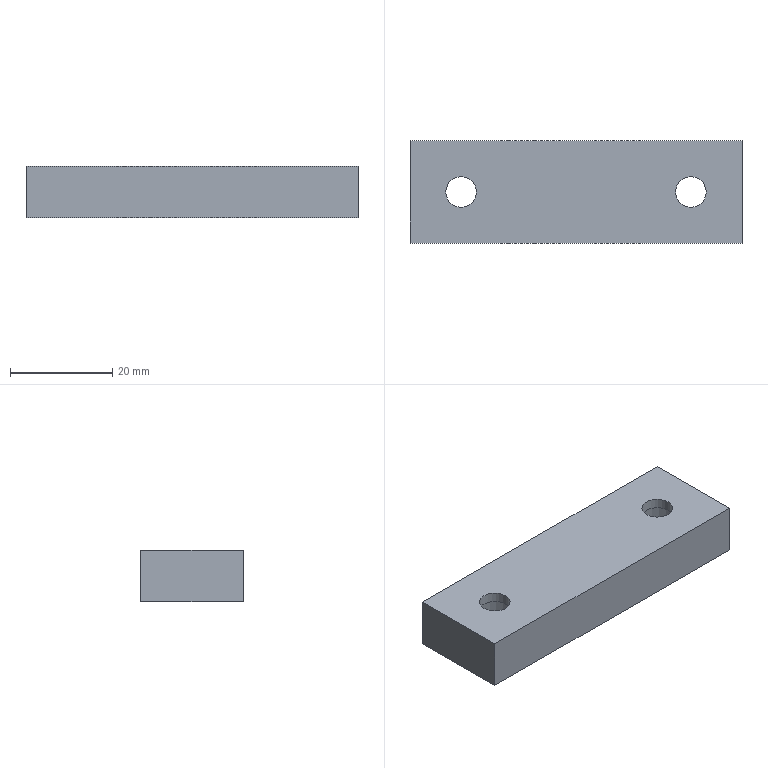Part | STEP file | gslz 2016.10.28-10_id2314_x_t | 1 solid | 12 faces | box 65 x 20 x 10 mm | volume 11366 mm3 | plane 8 | cylinder 4 | commonest cylinder face diameters 6 x2 11 x2
STEP:
#1=CARTESIAN_POINT('',(0.,0.,0.));
#2=DIRECTION('',(0.,0.,1.));
#3=DIRECTION('',(1.,0.,0.));
#4=AXIS2_PLACEMENT_3D('',#1,#2,#3);
#5=CARTESIAN_POINT('',(-56.5,250.,33.));
#6=VERTEX_POINT('',#5);
#7=CARTESIAN_POINT('',(-51.,250.,33.));
#8=DIRECTION('',(0.,0.,1.));
#9=DIRECTION('',(-1.,0.,0.));
#10=AXIS2_PLACEMENT_3D('',#7,#8,#9);
#11=CIRCLE('',#10,5.5);
#12=CARTESIAN_POINT('',(-51.,250.,35.));
#13=DIRECTION('',(0.,0.,-1.));
#14=DIRECTION('',(-1.,0.,0.));
#15=AXIS2_PLACEMENT_3D('',#12,#13,#14);
#16=CYLINDRICAL_SURFACE('',#15,5.5);
#17=CARTESIAN_POINT('',(6.283,2.));
#18=DIRECTION('',(-1.,0.));
#19=VECTOR('',#18,1.);
#20=LINE('',#17,#19);
#21=(GEOMETRIC_REPRESENTATION_CONTEXT(2)PARAMETRIC_REPRESENTATION_CONTEXT()REPRESENTATION_CONTEXT('',''));
#22=DEFINITIONAL_REPRESENTATION('',(#20),#21);
#23=PCURVE('',#16,#22);
#24=CARTESIAN_POINT('',(-13.5,250.,33.));
#25=DIRECTION('',(0.,0.,-1.));
#26=DIRECTION('',(1.,0.,0.));
#27=AXIS2_PLACEMENT_3D('',#24,#25,#26);
#28=PLANE('',#27);
#29=CARTESIAN_POINT('',(-43.,0.));
#30=CARTESIAN_POINT('',(-43.,9.526));
#31=CARTESIAN_POINT('',(-34.75,4.763));
#32=CARTESIAN_POINT('',(-26.5,0.));
#33=CARTESIAN_POINT('',(-34.75,-4.763));
#34=CARTESIAN_POINT('',(-43.,-9.526));
#35=CARTESIAN_POINT('',(-43.,0.));
#36=(BOUNDED_CURVE()B_SPLINE_CURVE(2,(#29,#30,#31,#32,#33,#34,#35),.UNSPECIFIED.,.T.,.F.)B_SPLINE_CURVE_WITH_KNOTS((1,2,2,2,2,1),(-2.094,0.,2.094,4.189,6.283,8.378),.UNSPECIFIED.)CURVE()GEOMETRIC_REPRESENTATION_ITEM()RATIONAL_B_SPLINE_CURVE((1.,0.5,1.,0.5,1.,0.5,1.))REPRESENTATION_ITEM(''));
#37=(GEOMETRIC_REPRESENTATION_CONTEXT(2)PARAMETRIC_REPRESENTATION_CONTEXT()REPRESENTATION_CONTEXT('',''));
#38=DEFINITIONAL_REPRESENTATION('',(#36),#37);
#39=PCURVE('',#28,#38);
#40=SURFACE_CURVE('',#11,(#23,#39),.PCURVE_S1.);
#41=EDGE_CURVE('',#6,#6,#40,.T.);
#42=ORIENTED_EDGE('',*,*,#41,.F.);
#43=CARTESIAN_POINT('',(-56.5,250.,25.));
#44=VERTEX_POINT('',#43);
#45=CARTESIAN_POINT('',(-56.5,250.,33.));
#46=CARTESIAN_POINT('',(-56.5,250.,25.));
#47=B_SPLINE_CURVE_WITH_KNOTS('',1,(#45,#46),.UNSPECIFIED.,.F.,.F.,(2,2),(2.,10.),.PIECEWISE_BEZIER_KNOTS.);
#48=CARTESIAN_POINT('',(6.283,0.));
#49=DIRECTION('',(0.,1.));
#50=VECTOR('',#49,1.);
#51=LINE('',#48,#50);
#52=(GEOMETRIC_REPRESENTATION_CONTEXT(2)PARAMETRIC_REPRESENTATION_CONTEXT()REPRESENTATION_CONTEXT('',''));
#53=DEFINITIONAL_REPRESENTATION('',(#51),#52);
#54=PCURVE('',#16,#53);
#55=CARTESIAN_POINT('',(0.,0.));
#56=DIRECTION('',(0.,1.));
#57=VECTOR('',#56,1.);
#58=LINE('',#55,#57);
#59=(GEOMETRIC_REPRESENTATION_CONTEXT(2)PARAMETRIC_REPRESENTATION_CONTEXT()REPRESENTATION_CONTEXT('',''));
#60=DEFINITIONAL_REPRESENTATION('',(#58),#59);
#61=PCURVE('',#16,#60);
#62=SEAM_CURVE('',#47,(#54,#61),.PCURVE_S1.);
#63=EDGE_CURVE('',#6,#44,#62,.T.);
#64=ORIENTED_EDGE('',*,*,#63,.T.);
#65=CARTESIAN_POINT('',(-45.5,250.,25.));
#66=VERTEX_POINT('',#65);
#67=CARTESIAN_POINT('',(-51.,250.,25.));
#68=DIRECTION('',(0.,0.,1.));
#69=DIRECTION('',(1.,0.,0.));
#70=AXIS2_PLACEMENT_3D('',#67,#68,#69);
#71=CIRCLE('',#70,5.5);
#72=CARTESIAN_POINT('',(9.425,10.));
#73=DIRECTION('',(-1.,0.));
#74=VECTOR('',#73,1.);
#75=LINE('',#72,#74);
#76=(GEOMETRIC_REPRESENTATION_CONTEXT(2)PARAMETRIC_REPRESENTATION_CONTEXT()REPRESENTATION_CONTEXT('',''));
#77=DEFINITIONAL_REPRESENTATION('',(#75),#76);
#78=PCURVE('',#16,#77);
#79=CARTESIAN_POINT('',(-98.5,250.,25.));
#80=DIRECTION('',(0.,0.,1.));
#81=DIRECTION('',(1.,0.,0.));
#82=AXIS2_PLACEMENT_3D('',#79,#80,#81);
#83=PLANE('',#82);
#84=CARTESIAN_POINT('',(47.5,0.));
#85=DIRECTION('',(1.,0.));
#86=AXIS2_PLACEMENT_2D('',#84,#85);
#87=CIRCLE('',#86,5.5);
#88=(GEOMETRIC_REPRESENTATION_CONTEXT(2)PARAMETRIC_REPRESENTATION_CONTEXT()REPRESENTATION_CONTEXT('',''));
#89=DEFINITIONAL_REPRESENTATION('',(#87),#88);
#90=PCURVE('',#83,#89);
#91=SURFACE_CURVE('',#71,(#78,#90),.PCURVE_S1.);
#92=EDGE_CURVE('',#44,#66,#91,.T.);
#93=ORIENTED_EDGE('',*,*,#92,.T.);
#94=CARTESIAN_POINT('',(-51.,250.,25.));
#95=DIRECTION('',(0.,0.,1.));
#96=DIRECTION('',(1.,0.,0.));
#97=AXIS2_PLACEMENT_3D('',#94,#95,#96);
#98=CIRCLE('',#97,5.5);
#99=CARTESIAN_POINT('',(3.142,10.));
#100=DIRECTION('',(-1.,0.));
#101=VECTOR('',#100,1.);
#102=LINE('',#99,#101);
#103=(GEOMETRIC_REPRESENTATION_CONTEXT(2)PARAMETRIC_REPRESENTATION_CONTEXT()REPRESENTATION_CONTEXT('',''));
#104=DEFINITIONAL_REPRESENTATION('',(#102),#103);
#105=PCURVE('',#16,#104);
#106=CARTESIAN_POINT('',(47.5,0.));
#107=DIRECTION('',(1.,0.));
#108=AXIS2_PLACEMENT_2D('',#106,#107);
#109=CIRCLE('',#108,5.5);
#110=(GEOMETRIC_REPRESENTATION_CONTEXT(2)PARAMETRIC_REPRESENTATION_CONTEXT()REPRESENTATION_CONTEXT('',''));
#111=DEFINITIONAL_REPRESENTATION('',(#109),#110);
#112=PCURVE('',#83,#111);
#113=SURFACE_CURVE('',#98,(#105,#112),.PCURVE_S1.);
#114=EDGE_CURVE('',#66,#44,#113,.T.);
#115=ORIENTED_EDGE('',*,*,#114,.T.);
#116=ORIENTED_EDGE('',*,*,#63,.F.);
#117=EDGE_LOOP('',(#42,#64,#93,#115,#116));
#118=FACE_BOUND('',#117,.F.);
#119=ADVANCED_FACE('',(#118),#16,.F.);
#120=CARTESIAN_POINT('',(-61.,260.,35.));
#121=VERTEX_POINT('',#120);
#122=CARTESIAN_POINT('',(-61.,260.,25.));
#123=VERTEX_POINT('',#122);
#124=CARTESIAN_POINT('',(-61.,260.,35.));
#125=DIRECTION('',(0.,0.,-1.));
#126=VECTOR('',#125,1.);
#127=LINE('',#124,#126);
#128=CARTESIAN_POINT('',(21.5,260.,35.));
#129=DIRECTION('',(0.,-1.,0.));
#130=DIRECTION('',(0.,0.,-1.));
#131=AXIS2_PLACEMENT_3D('',#128,#129,#130);
#132=PLANE('',#131);
#133=CARTESIAN_POINT('',(0.,-82.5));
#134=DIRECTION('',(1.,0.));
#135=VECTOR('',#134,1.);
#136=LINE('',#133,#135);
#137=(GEOMETRIC_REPRESENTATION_CONTEXT(2)PARAMETRIC_REPRESENTATION_CONTEXT()REPRESENTATION_CONTEXT('',''));
#138=DEFINITIONAL_REPRESENTATION('',(#136),#137);
#139=PCURVE('',#132,#138);
#140=CARTESIAN_POINT('',(-61.,262.5,35.));
#141=DIRECTION('',(1.,0.,0.));
#142=DIRECTION('',(0.,0.,-1.));
#143=AXIS2_PLACEMENT_3D('',#140,#141,#142);
#144=PLANE('',#143);
#145=CARTESIAN_POINT('',(0.,-2.5));
#146=DIRECTION('',(1.,0.));
#147=VECTOR('',#146,1.);
#148=LINE('',#145,#147);
#149=(GEOMETRIC_REPRESENTATION_CONTEXT(2)PARAMETRIC_REPRESENTATION_CONTEXT()REPRESENTATION_CONTEXT('',''));
#150=DEFINITIONAL_REPRESENTATION('',(#148),#149);
#151=PCURVE('',#144,#150);
#152=SURFACE_CURVE('',#127,(#139,#151),.PCURVE_S1.);
#153=EDGE_CURVE('',#121,#123,#152,.T.);
#154=ORIENTED_EDGE('',*,*,#153,.F.);
#155=CARTESIAN_POINT('',(4.,260.,35.));
#156=VERTEX_POINT('',#155);
#157=CARTESIAN_POINT('',(-98.5,260.,35.));
#158=DIRECTION('',(-1.,0.,0.));
#159=VECTOR('',#158,1.);
#160=LINE('',#157,#159);
#161=CARTESIAN_POINT('',(0.,-120.));
#162=DIRECTION('',(0.,-1.));
#163=VECTOR('',#162,1.);
#164=LINE('',#161,#163);
#165=(GEOMETRIC_REPRESENTATION_CONTEXT(2)PARAMETRIC_REPRESENTATION_CONTEXT()REPRESENTATION_CONTEXT('',''));
#166=DEFINITIONAL_REPRESENTATION('',(#164),#165);
#167=PCURVE('',#132,#166);
#168=CARTESIAN_POINT('',(-98.5,250.,35.));
#169=DIRECTION('',(0.,0.,1.));
#170=DIRECTION('',(1.,0.,0.));
#171=AXIS2_PLACEMENT_3D('',#168,#169,#170);
#172=PLANE('',#171);
#173=CARTESIAN_POINT('',(0.,10.));
#174=DIRECTION('',(-1.,0.));
#175=VECTOR('',#174,1.);
#176=LINE('',#173,#175);
#177=(GEOMETRIC_REPRESENTATION_CONTEXT(2)PARAMETRIC_REPRESENTATION_CONTEXT()REPRESENTATION_CONTEXT('',''));
#178=DEFINITIONAL_REPRESENTATION('',(#176),#177);
#179=PCURVE('',#172,#178);
#180=SURFACE_CURVE('',#160,(#167,#179),.PCURVE_S1.);
#181=EDGE_CURVE('',#156,#121,#180,.T.);
#182=ORIENTED_EDGE('',*,*,#181,.F.);
#183=CARTESIAN_POINT('',(4.,260.,25.));
#184=VERTEX_POINT('',#183);
#185=CARTESIAN_POINT('',(4.,260.,35.));
#186=DIRECTION('',(0.,0.,-1.));
#187=VECTOR('',#186,1.);
#188=LINE('',#185,#187);
#189=CARTESIAN_POINT('',(0.,-17.5));
#190=DIRECTION('',(1.,0.));
#191=VECTOR('',#190,1.);
#192=LINE('',#189,#191);
#193=(GEOMETRIC_REPRESENTATION_CONTEXT(2)PARAMETRIC_REPRESENTATION_CONTEXT()REPRESENTATION_CONTEXT('',''));
#194=DEFINITIONAL_REPRESENTATION('',(#192),#193);
#195=PCURVE('',#132,#194);
#196=CARTESIAN_POINT('',(4.,237.5,35.));
#197=DIRECTION('',(-1.,0.,0.));
#198=DIRECTION('',(0.,0.,1.));
#199=AXIS2_PLACEMENT_3D('',#196,#197,#198);
#200=PLANE('',#199);
#201=CARTESIAN_POINT('',(0.,22.5));
#202=DIRECTION('',(-1.,0.));
#203=VECTOR('',#202,1.);
#204=LINE('',#201,#203);
#205=(GEOMETRIC_REPRESENTATION_CONTEXT(2)PARAMETRIC_REPRESENTATION_CONTEXT()REPRESENTATION_CONTEXT('',''));
#206=DEFINITIONAL_REPRESENTATION('',(#204),#205);
#207=PCURVE('',#200,#206);
#208=SURFACE_CURVE('',#188,(#195,#207),.PCURVE_S1.);
#209=EDGE_CURVE('',#156,#184,#208,.T.);
#210=ORIENTED_EDGE('',*,*,#209,.T.);
#211=CARTESIAN_POINT('',(-98.5,260.,25.));
#212=DIRECTION('',(-1.,0.,0.));
#213=VECTOR('',#212,1.);
#214=LINE('',#211,#213);
#215=CARTESIAN_POINT('',(10.,-120.));
#216=DIRECTION('',(0.,-1.));
#217=VECTOR('',#216,1.);
#218=LINE('',#215,#217);
#219=(GEOMETRIC_REPRESENTATION_CONTEXT(2)PARAMETRIC_REPRESENTATION_CONTEXT()REPRESENTATION_CONTEXT('',''));
#220=DEFINITIONAL_REPRESENTATION('',(#218),#219);
#221=PCURVE('',#132,#220);
#222=CARTESIAN_POINT('',(0.,10.));
#223=DIRECTION('',(-1.,0.));
#224=VECTOR('',#223,1.);
#225=LINE('',#222,#224);
#226=(GEOMETRIC_REPRESENTATION_CONTEXT(2)PARAMETRIC_REPRESENTATION_CONTEXT()REPRESENTATION_CONTEXT('',''));
#227=DEFINITIONAL_REPRESENTATION('',(#225),#226);
#228=PCURVE('',#83,#227);
#229=SURFACE_CURVE('',#214,(#221,#228),.PCURVE_S1.);
#230=EDGE_CURVE('',#184,#123,#229,.T.);
#231=ORIENTED_EDGE('',*,*,#230,.T.);
#232=EDGE_LOOP('',(#154,#182,#210,#231));
#233=FACE_BOUND('',#232,.T.);
#234=ADVANCED_FACE('',(#233),#132,.F.);
#235=ORIENTED_EDGE('',*,*,#209,.F.);
#236=CARTESIAN_POINT('',(4.,240.,35.));
#237=VERTEX_POINT('',#236);
#238=CARTESIAN_POINT('',(4.,237.5,35.));
#239=DIRECTION('',(0.,1.,0.));
#240=VECTOR('',#239,1.);
#241=LINE('',#238,#240);
#242=CARTESIAN_POINT('',(0.,0.));
#243=DIRECTION('',(0.,1.));
#244=VECTOR('',#243,1.);
#245=LINE('',#242,#244);
#246=(GEOMETRIC_REPRESENTATION_CONTEXT(2)PARAMETRIC_REPRESENTATION_CONTEXT()REPRESENTATION_CONTEXT('',''));
#247=DEFINITIONAL_REPRESENTATION('',(#245),#246);
#248=PCURVE('',#200,#247);
#249=CARTESIAN_POINT('',(102.5,-12.5));
#250=DIRECTION('',(0.,1.));
#251=VECTOR('',#250,1.);
#252=LINE('',#249,#251);
#253=(GEOMETRIC_REPRESENTATION_CONTEXT(2)PARAMETRIC_REPRESENTATION_CONTEXT()REPRESENTATION_CONTEXT('',''));
#254=DEFINITIONAL_REPRESENTATION('',(#252),#253);
#255=PCURVE('',#172,#254);
#256=SURFACE_CURVE('',#241,(#248,#255),.PCURVE_S1.);
#257=EDGE_CURVE('',#237,#156,#256,.T.);
#258=ORIENTED_EDGE('',*,*,#257,.F.);
#259=CARTESIAN_POINT('',(4.,240.,25.));
#260=VERTEX_POINT('',#259);
#261=CARTESIAN_POINT('',(4.,240.,35.));
#262=DIRECTION('',(0.,0.,-1.));
#263=VECTOR('',#262,1.);
#264=LINE('',#261,#263);
#265=CARTESIAN_POINT('',(0.,2.5));
#266=DIRECTION('',(-1.,0.));
#267=VECTOR('',#266,1.);
#268=LINE('',#265,#267);
#269=(GEOMETRIC_REPRESENTATION_CONTEXT(2)PARAMETRIC_REPRESENTATION_CONTEXT()REPRESENTATION_CONTEXT('',''));
#270=DEFINITIONAL_REPRESENTATION('',(#268),#269);
#271=PCURVE('',#200,#270);
#272=CARTESIAN_POINT('',(-108.5,240.,35.));
#273=DIRECTION('',(0.,1.,0.));
#274=DIRECTION('',(0.,0.,1.));
#275=AXIS2_PLACEMENT_3D('',#272,#273,#274);
#276=PLANE('',#275);
#277=CARTESIAN_POINT('',(0.,112.5));
#278=DIRECTION('',(-1.,0.));
#279=VECTOR('',#278,1.);
#280=LINE('',#277,#279);
#281=(GEOMETRIC_REPRESENTATION_CONTEXT(2)PARAMETRIC_REPRESENTATION_CONTEXT()REPRESENTATION_CONTEXT('',''));
#282=DEFINITIONAL_REPRESENTATION('',(#280),#281);
#283=PCURVE('',#276,#282);
#284=SURFACE_CURVE('',#264,(#271,#283),.PCURVE_S1.);
#285=EDGE_CURVE('',#237,#260,#284,.T.);
#286=ORIENTED_EDGE('',*,*,#285,.T.);
#287=CARTESIAN_POINT('',(4.,237.5,25.));
#288=DIRECTION('',(0.,1.,0.));
#289=VECTOR('',#288,1.);
#290=LINE('',#287,#289);
#291=CARTESIAN_POINT('',(-10.,0.));
#292=DIRECTION('',(0.,1.));
#293=VECTOR('',#292,1.);
#294=LINE('',#291,#293);
#295=(GEOMETRIC_REPRESENTATION_CONTEXT(2)PARAMETRIC_REPRESENTATION_CONTEXT()REPRESENTATION_CONTEXT('',''));
#296=DEFINITIONAL_REPRESENTATION('',(#294),#295);
#297=PCURVE('',#200,#296);
#298=CARTESIAN_POINT('',(102.5,-12.5));
#299=DIRECTION('',(0.,1.));
#300=VECTOR('',#299,1.);
#301=LINE('',#298,#300);
#302=(GEOMETRIC_REPRESENTATION_CONTEXT(2)PARAMETRIC_REPRESENTATION_CONTEXT()REPRESENTATION_CONTEXT('',''));
#303=DEFINITIONAL_REPRESENTATION('',(#301),#302);
#304=PCURVE('',#83,#303);
#305=SURFACE_CURVE('',#290,(#297,#304),.PCURVE_S1.);
#306=EDGE_CURVE('',#260,#184,#305,.T.);
#307=ORIENTED_EDGE('',*,*,#306,.T.);
#308=EDGE_LOOP('',(#235,#258,#286,#307));
#309=FACE_BOUND('',#308,.T.);
#310=ADVANCED_FACE('',(#309),#200,.F.);
#311=ORIENTED_EDGE('',*,*,#285,.F.);
#312=CARTESIAN_POINT('',(-61.,240.,35.));
#313=VERTEX_POINT('',#312);
#314=CARTESIAN_POINT('',(-98.5,240.,35.));
#315=DIRECTION('',(1.,0.,0.));
#316=VECTOR('',#315,1.);
#317=LINE('',#314,#316);
#318=CARTESIAN_POINT('',(0.,10.));
#319=DIRECTION('',(0.,1.));
#320=VECTOR('',#319,1.);
#321=LINE('',#318,#320);
#322=(GEOMETRIC_REPRESENTATION_CONTEXT(2)PARAMETRIC_REPRESENTATION_CONTEXT()REPRESENTATION_CONTEXT('',''));
#323=DEFINITIONAL_REPRESENTATION('',(#321),#322);
#324=PCURVE('',#276,#323);
#325=CARTESIAN_POINT('',(0.,-10.));
#326=DIRECTION('',(1.,0.));
#327=VECTOR('',#326,1.);
#328=LINE('',#325,#327);
#329=(GEOMETRIC_REPRESENTATION_CONTEXT(2)PARAMETRIC_REPRESENTATION_CONTEXT()REPRESENTATION_CONTEXT('',''));
#330=DEFINITIONAL_REPRESENTATION('',(#328),#329);
#331=PCURVE('',#172,#330);
#332=SURFACE_CURVE('',#317,(#324,#331),.PCURVE_S1.);
#333=EDGE_CURVE('',#313,#237,#332,.T.);
#334=ORIENTED_EDGE('',*,*,#333,.F.);
#335=CARTESIAN_POINT('',(-61.,240.,25.));
#336=VERTEX_POINT('',#335);
#337=CARTESIAN_POINT('',(-61.,240.,35.));
#338=DIRECTION('',(0.,0.,-1.));
#339=VECTOR('',#338,1.);
#340=LINE('',#337,#339);
#341=CARTESIAN_POINT('',(0.,47.5));
#342=DIRECTION('',(-1.,0.));
#343=VECTOR('',#342,1.);
#344=LINE('',#341,#343);
#345=(GEOMETRIC_REPRESENTATION_CONTEXT(2)PARAMETRIC_REPRESENTATION_CONTEXT()REPRESENTATION_CONTEXT('',''));
#346=DEFINITIONAL_REPRESENTATION('',(#344),#345);
#347=PCURVE('',#276,#346);
#348=CARTESIAN_POINT('',(0.,-22.5));
#349=DIRECTION('',(1.,0.));
#350=VECTOR('',#349,1.);
#351=LINE('',#348,#350);
#352=(GEOMETRIC_REPRESENTATION_CONTEXT(2)PARAMETRIC_REPRESENTATION_CONTEXT()REPRESENTATION_CONTEXT('',''));
#353=DEFINITIONAL_REPRESENTATION('',(#351),#352);
#354=PCURVE('',#144,#353);
#355=SURFACE_CURVE('',#340,(#347,#354),.PCURVE_S1.);
#356=EDGE_CURVE('',#313,#336,#355,.T.);
#357=ORIENTED_EDGE('',*,*,#356,.T.);
#358=CARTESIAN_POINT('',(-98.5,240.,25.));
#359=DIRECTION('',(1.,0.,0.));
#360=VECTOR('',#359,1.);
#361=LINE('',#358,#360);
#362=CARTESIAN_POINT('',(-10.,10.));
#363=DIRECTION('',(0.,1.));
#364=VECTOR('',#363,1.);
#365=LINE('',#362,#364);
#366=(GEOMETRIC_REPRESENTATION_CONTEXT(2)PARAMETRIC_REPRESENTATION_CONTEXT()REPRESENTATION_CONTEXT('',''));
#367=DEFINITIONAL_REPRESENTATION('',(#365),#366);
#368=PCURVE('',#276,#367);
#369=CARTESIAN_POINT('',(0.,-10.));
#370=DIRECTION('',(1.,0.));
#371=VECTOR('',#370,1.);
#372=LINE('',#369,#371);
#373=(GEOMETRIC_REPRESENTATION_CONTEXT(2)PARAMETRIC_REPRESENTATION_CONTEXT()REPRESENTATION_CONTEXT('',''));
#374=DEFINITIONAL_REPRESENTATION('',(#372),#373);
#375=PCURVE('',#83,#374);
#376=SURFACE_CURVE('',#361,(#368,#375),.PCURVE_S1.);
#377=EDGE_CURVE('',#336,#260,#376,.T.);
#378=ORIENTED_EDGE('',*,*,#377,.T.);
#379=EDGE_LOOP('',(#311,#334,#357,#378));
#380=FACE_BOUND('',#379,.T.);
#381=ADVANCED_FACE('',(#380),#276,.F.);
#382=ORIENTED_EDGE('',*,*,#356,.F.);
#383=CARTESIAN_POINT('',(-61.,262.5,35.));
#384=DIRECTION('',(0.,-1.,0.));
#385=VECTOR('',#384,1.);
#386=LINE('',#383,#385);
#387=CARTESIAN_POINT('',(0.,0.));
#388=DIRECTION('',(0.,-1.));
#389=VECTOR('',#388,1.);
#390=LINE('',#387,#389);
#391=(GEOMETRIC_REPRESENTATION_CONTEXT(2)PARAMETRIC_REPRESENTATION_CONTEXT()REPRESENTATION_CONTEXT('',''));
#392=DEFINITIONAL_REPRESENTATION('',(#390),#391);
#393=PCURVE('',#144,#392);
#394=CARTESIAN_POINT('',(37.5,12.5));
#395=DIRECTION('',(0.,-1.));
#396=VECTOR('',#395,1.);
#397=LINE('',#394,#396);
#398=(GEOMETRIC_REPRESENTATION_CONTEXT(2)PARAMETRIC_REPRESENTATION_CONTEXT()REPRESENTATION_CONTEXT('',''));
#399=DEFINITIONAL_REPRESENTATION('',(#397),#398);
#400=PCURVE('',#172,#399);
#401=SURFACE_CURVE('',#386,(#393,#400),.PCURVE_S1.);
#402=EDGE_CURVE('',#121,#313,#401,.T.);
#403=ORIENTED_EDGE('',*,*,#402,.F.);
#404=ORIENTED_EDGE('',*,*,#153,.T.);
#405=CARTESIAN_POINT('',(-61.,262.5,25.));
#406=DIRECTION('',(0.,-1.,0.));
#407=VECTOR('',#406,1.);
#408=LINE('',#405,#407);
#409=CARTESIAN_POINT('',(10.,0.));
#410=DIRECTION('',(0.,-1.));
#411=VECTOR('',#410,1.);
#412=LINE('',#409,#411);
#413=(GEOMETRIC_REPRESENTATION_CONTEXT(2)PARAMETRIC_REPRESENTATION_CONTEXT()REPRESENTATION_CONTEXT('',''));
#414=DEFINITIONAL_REPRESENTATION('',(#412),#413);
#415=PCURVE('',#144,#414);
#416=CARTESIAN_POINT('',(37.5,12.5));
#417=DIRECTION('',(0.,-1.));
#418=VECTOR('',#417,1.);
#419=LINE('',#416,#418);
#420=(GEOMETRIC_REPRESENTATION_CONTEXT(2)PARAMETRIC_REPRESENTATION_CONTEXT()REPRESENTATION_CONTEXT('',''));
#421=DEFINITIONAL_REPRESENTATION('',(#419),#420);
#422=PCURVE('',#83,#421);
#423=SURFACE_CURVE('',#408,(#415,#422),.PCURVE_S1.);
#424=EDGE_CURVE('',#123,#336,#423,.T.);
#425=ORIENTED_EDGE('',*,*,#424,.T.);
#426=EDGE_LOOP('',(#382,#403,#404,#425));
#427=FACE_BOUND('',#426,.T.);
#428=ADVANCED_FACE('',(#427),#144,.F.);
#429=ORIENTED_EDGE('',*,*,#424,.F.);
#430=ORIENTED_EDGE('',*,*,#230,.F.);
#431=ORIENTED_EDGE('',*,*,#306,.F.);
#432=ORIENTED_EDGE('',*,*,#377,.F.);
#433=EDGE_LOOP('',(#429,#430,#431,#432));
#434=FACE_BOUND('',#433,.T.);
#435=ORIENTED_EDGE('',*,*,#114,.T.);
#436=ORIENTED_EDGE('',*,*,#92,.T.);
#437=EDGE_LOOP('',(#435,#436));
#438=FACE_BOUND('',#437,.T.);
#439=CARTESIAN_POINT('',(-0.5,250.,25.));
#440=VERTEX_POINT('',#439);
#441=CARTESIAN_POINT('',(-11.5,250.,25.));
#442=VERTEX_POINT('',#441);
#443=CARTESIAN_POINT('',(-6.,250.,25.));
#444=DIRECTION('',(0.,0.,1.));
#445=DIRECTION('',(1.,0.,0.));
#446=AXIS2_PLACEMENT_3D('',#443,#444,#445);
#447=CIRCLE('',#446,5.5);
#448=CARTESIAN_POINT('',(92.5,0.));
#449=DIRECTION('',(1.,0.));
#450=AXIS2_PLACEMENT_2D('',#448,#449);
#451=CIRCLE('',#450,5.5);
#452=(GEOMETRIC_REPRESENTATION_CONTEXT(2)PARAMETRIC_REPRESENTATION_CONTEXT()REPRESENTATION_CONTEXT('',''));
#453=DEFINITIONAL_REPRESENTATION('',(#451),#452);
#454=PCURVE('',#83,#453);
#455=CARTESIAN_POINT('',(-6.,250.,35.));
#456=DIRECTION('',(0.,0.,-1.));
#457=DIRECTION('',(-1.,0.,0.));
#458=AXIS2_PLACEMENT_3D('',#455,#456,#457);
#459=CYLINDRICAL_SURFACE('',#458,5.5);
#460=CARTESIAN_POINT('',(3.142,10.));
#461=DIRECTION('',(-1.,0.));
#462=VECTOR('',#461,1.);
#463=LINE('',#460,#462);
#464=(GEOMETRIC_REPRESENTATION_CONTEXT(2)PARAMETRIC_REPRESENTATION_CONTEXT()REPRESENTATION_CONTEXT('',''));
#465=DEFINITIONAL_REPRESENTATION('',(#463),#464);
#466=PCURVE('',#459,#465);
#467=SURFACE_CURVE('',#447,(#454,#466),.PCURVE_S1.);
#468=EDGE_CURVE('',#440,#442,#467,.T.);
#469=ORIENTED_EDGE('',*,*,#468,.T.);
#470=CARTESIAN_POINT('',(-6.,250.,25.));
#471=DIRECTION('',(0.,0.,1.));
#472=DIRECTION('',(1.,0.,0.));
#473=AXIS2_PLACEMENT_3D('',#470,#471,#472);
#474=CIRCLE('',#473,5.5);
#475=CARTESIAN_POINT('',(92.5,0.));
#476=DIRECTION('',(1.,0.));
#477=AXIS2_PLACEMENT_2D('',#475,#476);
#478=CIRCLE('',#477,5.5);
#479=(GEOMETRIC_REPRESENTATION_CONTEXT(2)PARAMETRIC_REPRESENTATION_CONTEXT()REPRESENTATION_CONTEXT('',''));
#480=DEFINITIONAL_REPRESENTATION('',(#478),#479);
#481=PCURVE('',#83,#480);
#482=CARTESIAN_POINT('',(9.425,10.));
#483=DIRECTION('',(-1.,0.));
#484=VECTOR('',#483,1.);
#485=LINE('',#482,#484);
#486=(GEOMETRIC_REPRESENTATION_CONTEXT(2)PARAMETRIC_REPRESENTATION_CONTEXT()REPRESENTATION_CONTEXT('',''));
#487=DEFINITIONAL_REPRESENTATION('',(#485),#486);
#488=PCURVE('',#459,#487);
#489=SURFACE_CURVE('',#474,(#481,#488),.PCURVE_S1.);
#490=EDGE_CURVE('',#442,#440,#489,.T.);
#491=ORIENTED_EDGE('',*,*,#490,.T.);
#492=EDGE_LOOP('',(#469,#491));
#493=FACE_BOUND('',#492,.T.);
#494=ADVANCED_FACE('',(#434,#438,#493),#83,.F.);
#495=CARTESIAN_POINT('',(-11.5,250.,33.));
#496=VERTEX_POINT('',#495);
#497=CARTESIAN_POINT('',(-6.,250.,33.));
#498=DIRECTION('',(0.,0.,1.));
#499=DIRECTION('',(-1.,0.,0.));
#500=AXIS2_PLACEMENT_3D('',#497,#498,#499);
#501=CIRCLE('',#500,5.5);
#502=CARTESIAN_POINT('',(6.283,2.));
#503=DIRECTION('',(-1.,0.));
#504=VECTOR('',#503,1.);
#505=LINE('',#502,#504);
#506=(GEOMETRIC_REPRESENTATION_CONTEXT(2)PARAMETRIC_REPRESENTATION_CONTEXT()REPRESENTATION_CONTEXT('',''));
#507=DEFINITIONAL_REPRESENTATION('',(#505),#506);
#508=PCURVE('',#459,#507);
#509=CARTESIAN_POINT('',(-43.5,250.,33.));
#510=DIRECTION('',(0.,0.,-1.));
#511=DIRECTION('',(1.,0.,0.));
#512=AXIS2_PLACEMENT_3D('',#509,#510,#511);
#513=PLANE('',#512);
#514=CARTESIAN_POINT('',(32.,0.));
#515=CARTESIAN_POINT('',(32.,9.526));
#516=CARTESIAN_POINT('',(40.25,4.763));
#517=CARTESIAN_POINT('',(48.5,0.));
#518=CARTESIAN_POINT('',(40.25,-4.763));
#519=CARTESIAN_POINT('',(32.,-9.526));
#520=CARTESIAN_POINT('',(32.,0.));
#521=(BOUNDED_CURVE()B_SPLINE_CURVE(2,(#514,#515,#516,#517,#518,#519,#520),.UNSPECIFIED.,.T.,.F.)B_SPLINE_CURVE_WITH_KNOTS((1,2,2,2,2,1),(-2.094,0.,2.094,4.189,6.283,8.378),.UNSPECIFIED.)CURVE()GEOMETRIC_REPRESENTATION_ITEM()RATIONAL_B_SPLINE_CURVE((1.,0.5,1.,0.5,1.,0.5,1.))REPRESENTATION_ITEM(''));
#522=(GEOMETRIC_REPRESENTATION_CONTEXT(2)PARAMETRIC_REPRESENTATION_CONTEXT()REPRESENTATION_CONTEXT('',''));
#523=DEFINITIONAL_REPRESENTATION('',(#521),#522);
#524=PCURVE('',#513,#523);
#525=SURFACE_CURVE('',#501,(#508,#524),.PCURVE_S1.);
#526=EDGE_CURVE('',#496,#496,#525,.T.);
#527=ORIENTED_EDGE('',*,*,#526,.F.);
#528=CARTESIAN_POINT('',(-11.5,250.,33.));
#529=CARTESIAN_POINT('',(-11.5,250.,25.));
#530=B_SPLINE_CURVE_WITH_KNOTS('',1,(#528,#529),.UNSPECIFIED.,.F.,.F.,(2,2),(2.,10.),.PIECEWISE_BEZIER_KNOTS.);
#531=CARTESIAN_POINT('',(6.283,0.));
#532=DIRECTION('',(0.,1.));
#533=VECTOR('',#532,1.);
#534=LINE('',#531,#533);
#535=(GEOMETRIC_REPRESENTATION_CONTEXT(2)PARAMETRIC_REPRESENTATION_CONTEXT()REPRESENTATION_CONTEXT('',''));
#536=DEFINITIONAL_REPRESENTATION('',(#534),#535);
#537=PCURVE('',#459,#536);
#538=CARTESIAN_POINT('',(0.,0.));
#539=DIRECTION('',(0.,1.));
#540=VECTOR('',#539,1.);
#541=LINE('',#538,#540);
#542=(GEOMETRIC_REPRESENTATION_CONTEXT(2)PARAMETRIC_REPRESENTATION_CONTEXT()REPRESENTATION_CONTEXT('',''));
#543=DEFINITIONAL_REPRESENTATION('',(#541),#542);
#544=PCURVE('',#459,#543);
#545=SEAM_CURVE('',#530,(#537,#544),.PCURVE_S1.);
#546=EDGE_CURVE('',#496,#442,#545,.T.);
#547=ORIENTED_EDGE('',*,*,#546,.T.);
#548=ORIENTED_EDGE('',*,*,#490,.T.);
#549=ORIENTED_EDGE('',*,*,#468,.T.);
#550=ORIENTED_EDGE('',*,*,#546,.F.);
#551=EDGE_LOOP('',(#527,#547,#548,#549,#550));
#552=FACE_BOUND('',#551,.F.);
#553=ADVANCED_FACE('',(#552),#459,.F.);
#554=CARTESIAN_POINT('',(-9.,250.,33.));
#555=VERTEX_POINT('',#554);
#556=CARTESIAN_POINT('',(-6.,250.,33.));
#557=DIRECTION('',(0.,0.,-1.));
#558=DIRECTION('',(-1.,0.,0.));
#559=AXIS2_PLACEMENT_3D('',#556,#557,#558);
#560=CIRCLE('',#559,3.);
#561=CARTESIAN_POINT('',(37.5,0.));
#562=DIRECTION('',(-1.,0.));
#563=AXIS2_PLACEMENT_2D('',#561,#562);
#564=CIRCLE('',#563,3.);
#565=(GEOMETRIC_REPRESENTATION_CONTEXT(2)PARAMETRIC_REPRESENTATION_CONTEXT()REPRESENTATION_CONTEXT('',''));
#566=DEFINITIONAL_REPRESENTATION('',(#564),#565);
#567=PCURVE('',#513,#566);
#568=CARTESIAN_POINT('',(-6.,250.,35.));
#569=DIRECTION('',(0.,0.,-1.));
#570=DIRECTION('',(-1.,0.,0.));
#571=AXIS2_PLACEMENT_3D('',#568,#569,#570);
#572=CYLINDRICAL_SURFACE('',#571,3.);
#573=CARTESIAN_POINT('',(0.,2.));
#574=DIRECTION('',(1.,0.));
#575=VECTOR('',#574,1.);
#576=LINE('',#573,#575);
#577=(GEOMETRIC_REPRESENTATION_CONTEXT(2)PARAMETRIC_REPRESENTATION_CONTEXT()REPRESENTATION_CONTEXT('',''));
#578=DEFINITIONAL_REPRESENTATION('',(#576),#577);
#579=PCURVE('',#572,#578);
#580=SURFACE_CURVE('',#560,(#567,#579),.PCURVE_S1.);
#581=EDGE_CURVE('',#555,#555,#580,.T.);
#582=ORIENTED_EDGE('',*,*,#581,.F.);
#583=EDGE_LOOP('',(#582));
#584=FACE_BOUND('',#583,.T.);
#585=ORIENTED_EDGE('',*,*,#526,.F.);
#586=EDGE_LOOP('',(#585));
#587=FACE_BOUND('',#586,.T.);
#588=ADVANCED_FACE('',(#584,#587),#513,.T.);
#589=CARTESIAN_POINT('',(-54.,250.,33.));
#590=VERTEX_POINT('',#589);
#591=CARTESIAN_POINT('',(-51.,250.,33.));
#592=DIRECTION('',(0.,0.,-1.));
#593=DIRECTION('',(-1.,0.,0.));
#594=AXIS2_PLACEMENT_3D('',#591,#592,#593);
#595=CIRCLE('',#594,3.);
#596=CARTESIAN_POINT('',(-37.5,0.));
#597=DIRECTION('',(-1.,0.));
#598=AXIS2_PLACEMENT_2D('',#596,#597);
#599=CIRCLE('',#598,3.);
#600=(GEOMETRIC_REPRESENTATION_CONTEXT(2)PARAMETRIC_REPRESENTATION_CONTEXT()REPRESENTATION_CONTEXT('',''));
#601=DEFINITIONAL_REPRESENTATION('',(#599),#600);
#602=PCURVE('',#28,#601);
#603=CARTESIAN_POINT('',(-51.,250.,35.));
#604=DIRECTION('',(0.,0.,-1.));
#605=DIRECTION('',(-1.,0.,0.));
#606=AXIS2_PLACEMENT_3D('',#603,#604,#605);
#607=CYLINDRICAL_SURFACE('',#606,3.);
#608=CARTESIAN_POINT('',(0.,2.));
#609=DIRECTION('',(1.,0.));
#610=VECTOR('',#609,1.);
#611=LINE('',#608,#610);
#612=(GEOMETRIC_REPRESENTATION_CONTEXT(2)PARAMETRIC_REPRESENTATION_CONTEXT()REPRESENTATION_CONTEXT('',''));
#613=DEFINITIONAL_REPRESENTATION('',(#611),#612);
#614=PCURVE('',#607,#613);
#615=SURFACE_CURVE('',#595,(#602,#614),.PCURVE_S1.);
#616=EDGE_CURVE('',#590,#590,#615,.T.);
#617=ORIENTED_EDGE('',*,*,#616,.F.);
#618=EDGE_LOOP('',(#617));
#619=FACE_BOUND('',#618,.T.);
#620=ORIENTED_EDGE('',*,*,#41,.F.);
#621=EDGE_LOOP('',(#620));
#622=FACE_BOUND('',#621,.T.);
#623=ADVANCED_FACE('',(#619,#622),#28,.T.);
#624=CARTESIAN_POINT('',(-54.,250.,35.));
#625=VERTEX_POINT('',#624);
#626=CARTESIAN_POINT('',(-48.,250.,35.));
#627=VERTEX_POINT('',#626);
#628=CARTESIAN_POINT('',(-51.,250.,35.));
#629=DIRECTION('',(0.,0.,1.));
#630=DIRECTION('',(1.,0.,0.));
#631=AXIS2_PLACEMENT_3D('',#628,#629,#630);
#632=CIRCLE('',#631,3.);
#633=CARTESIAN_POINT('',(9.425,0.));
#634=DIRECTION('',(-1.,0.));
#635=VECTOR('',#634,1.);
#636=LINE('',#633,#635);
#637=(GEOMETRIC_REPRESENTATION_CONTEXT(2)PARAMETRIC_REPRESENTATION_CONTEXT()REPRESENTATION_CONTEXT('',''));
#638=DEFINITIONAL_REPRESENTATION('',(#636),#637);
#639=PCURVE('',#607,#638);
#640=CARTESIAN_POINT('',(47.5,0.));
#641=DIRECTION('',(1.,0.));
#642=AXIS2_PLACEMENT_2D('',#640,#641);
#643=CIRCLE('',#642,3.);
#644=(GEOMETRIC_REPRESENTATION_CONTEXT(2)PARAMETRIC_REPRESENTATION_CONTEXT()REPRESENTATION_CONTEXT('',''));
#645=DEFINITIONAL_REPRESENTATION('',(#643),#644);
#646=PCURVE('',#172,#645);
#647=SURFACE_CURVE('',#632,(#639,#646),.PCURVE_S1.);
#648=EDGE_CURVE('',#625,#627,#647,.T.);
#649=ORIENTED_EDGE('',*,*,#648,.F.);
#650=CARTESIAN_POINT('',(-54.,250.,35.));
#651=CARTESIAN_POINT('',(-54.,250.,33.));
#652=B_SPLINE_CURVE_WITH_KNOTS('',1,(#650,#651),.UNSPECIFIED.,.F.,.F.,(2,2),(0.,2.),.PIECEWISE_BEZIER_KNOTS.);
#653=CARTESIAN_POINT('',(6.283,0.));
#654=DIRECTION('',(0.,1.));
#655=VECTOR('',#654,1.);
#656=LINE('',#653,#655);
#657=(GEOMETRIC_REPRESENTATION_CONTEXT(2)PARAMETRIC_REPRESENTATION_CONTEXT()REPRESENTATION_CONTEXT('',''));
#658=DEFINITIONAL_REPRESENTATION('',(#656),#657);
#659=PCURVE('',#607,#658);
#660=CARTESIAN_POINT('',(0.,0.));
#661=DIRECTION('',(0.,1.));
#662=VECTOR('',#661,1.);
#663=LINE('',#660,#662);
#664=(GEOMETRIC_REPRESENTATION_CONTEXT(2)PARAMETRIC_REPRESENTATION_CONTEXT()REPRESENTATION_CONTEXT('',''));
#665=DEFINITIONAL_REPRESENTATION('',(#663),#664);
#666=PCURVE('',#607,#665);
#667=SEAM_CURVE('',#652,(#659,#666),.PCURVE_S1.);
#668=EDGE_CURVE('',#625,#590,#667,.T.);
#669=ORIENTED_EDGE('',*,*,#668,.T.);
#670=ORIENTED_EDGE('',*,*,#616,.F.);
#671=ORIENTED_EDGE('',*,*,#668,.F.);
#672=CARTESIAN_POINT('',(-51.,250.,35.));
#673=DIRECTION('',(0.,0.,1.));
#674=DIRECTION('',(1.,0.,0.));
#675=AXIS2_PLACEMENT_3D('',#672,#673,#674);
#676=CIRCLE('',#675,3.);
#677=CARTESIAN_POINT('',(3.142,0.));
#678=DIRECTION('',(-1.,0.));
#679=VECTOR('',#678,1.);
#680=LINE('',#677,#679);
#681=(GEOMETRIC_REPRESENTATION_CONTEXT(2)PARAMETRIC_REPRESENTATION_CONTEXT()REPRESENTATION_CONTEXT('',''));
#682=DEFINITIONAL_REPRESENTATION('',(#680),#681);
#683=PCURVE('',#607,#682);
#684=CARTESIAN_POINT('',(47.5,0.));
#685=DIRECTION('',(1.,0.));
#686=AXIS2_PLACEMENT_2D('',#684,#685);
#687=CIRCLE('',#686,3.);
#688=(GEOMETRIC_REPRESENTATION_CONTEXT(2)PARAMETRIC_REPRESENTATION_CONTEXT()REPRESENTATION_CONTEXT('',''));
#689=DEFINITIONAL_REPRESENTATION('',(#687),#688);
#690=PCURVE('',#172,#689);
#691=SURFACE_CURVE('',#676,(#683,#690),.PCURVE_S1.);
#692=EDGE_CURVE('',#627,#625,#691,.T.);
#693=ORIENTED_EDGE('',*,*,#692,.F.);
#694=EDGE_LOOP('',(#649,#669,#670,#671,#693));
#695=FACE_BOUND('',#694,.F.);
#696=ADVANCED_FACE('',(#695),#607,.F.);
#697=CARTESIAN_POINT('',(-9.,250.,35.));
#698=VERTEX_POINT('',#697);
#699=CARTESIAN_POINT('',(-3.,250.,35.));
#700=VERTEX_POINT('',#699);
#701=CARTESIAN_POINT('',(-6.,250.,35.));
#702=DIRECTION('',(0.,0.,1.));
#703=DIRECTION('',(1.,0.,0.));
#704=AXIS2_PLACEMENT_3D('',#701,#702,#703);
#705=CIRCLE('',#704,3.);
#706=CARTESIAN_POINT('',(9.425,0.));
#707=DIRECTION('',(-1.,0.));
#708=VECTOR('',#707,1.);
#709=LINE('',#706,#708);
#710=(GEOMETRIC_REPRESENTATION_CONTEXT(2)PARAMETRIC_REPRESENTATION_CONTEXT()REPRESENTATION_CONTEXT('',''));
#711=DEFINITIONAL_REPRESENTATION('',(#709),#710);
#712=PCURVE('',#572,#711);
#713=CARTESIAN_POINT('',(92.5,0.));
#714=DIRECTION('',(1.,0.));
#715=AXIS2_PLACEMENT_2D('',#713,#714);
#716=CIRCLE('',#715,3.);
#717=(GEOMETRIC_REPRESENTATION_CONTEXT(2)PARAMETRIC_REPRESENTATION_CONTEXT()REPRESENTATION_CONTEXT('',''));
#718=DEFINITIONAL_REPRESENTATION('',(#716),#717);
#719=PCURVE('',#172,#718);
#720=SURFACE_CURVE('',#705,(#712,#719),.PCURVE_S1.);
#721=EDGE_CURVE('',#698,#700,#720,.T.);
#722=ORIENTED_EDGE('',*,*,#721,.F.);
#723=CARTESIAN_POINT('',(-9.,250.,35.));
#724=CARTESIAN_POINT('',(-9.,250.,33.));
#725=B_SPLINE_CURVE_WITH_KNOTS('',1,(#723,#724),.UNSPECIFIED.,.F.,.F.,(2,2),(0.,2.),.PIECEWISE_BEZIER_KNOTS.);
#726=CARTESIAN_POINT('',(6.283,0.));
#727=DIRECTION('',(0.,1.));
#728=VECTOR('',#727,1.);
#729=LINE('',#726,#728);
#730=(GEOMETRIC_REPRESENTATION_CONTEXT(2)PARAMETRIC_REPRESENTATION_CONTEXT()REPRESENTATION_CONTEXT('',''));
#731=DEFINITIONAL_REPRESENTATION('',(#729),#730);
#732=PCURVE('',#572,#731);
#733=CARTESIAN_POINT('',(0.,0.));
#734=DIRECTION('',(0.,1.));
#735=VECTOR('',#734,1.);
#736=LINE('',#733,#735);
#737=(GEOMETRIC_REPRESENTATION_CONTEXT(2)PARAMETRIC_REPRESENTATION_CONTEXT()REPRESENTATION_CONTEXT('',''));
#738=DEFINITIONAL_REPRESENTATION('',(#736),#737);
#739=PCURVE('',#572,#738);
#740=SEAM_CURVE('',#725,(#732,#739),.PCURVE_S1.);
#741=EDGE_CURVE('',#698,#555,#740,.T.);
#742=ORIENTED_EDGE('',*,*,#741,.T.);
#743=ORIENTED_EDGE('',*,*,#581,.F.);
#744=ORIENTED_EDGE('',*,*,#741,.F.);
#745=CARTESIAN_POINT('',(-6.,250.,35.));
#746=DIRECTION('',(0.,0.,1.));
#747=DIRECTION('',(1.,0.,0.));
#748=AXIS2_PLACEMENT_3D('',#745,#746,#747);
#749=CIRCLE('',#748,3.);
#750=CARTESIAN_POINT('',(3.142,0.));
#751=DIRECTION('',(-1.,0.));
#752=VECTOR('',#751,1.);
#753=LINE('',#750,#752);
#754=(GEOMETRIC_REPRESENTATION_CONTEXT(2)PARAMETRIC_REPRESENTATION_CONTEXT()REPRESENTATION_CONTEXT('',''));
#755=DEFINITIONAL_REPRESENTATION('',(#753),#754);
#756=PCURVE('',#572,#755);
#757=CARTESIAN_POINT('',(92.5,0.));
#758=DIRECTION('',(1.,0.));
#759=AXIS2_PLACEMENT_2D('',#757,#758);
#760=CIRCLE('',#759,3.);
#761=(GEOMETRIC_REPRESENTATION_CONTEXT(2)PARAMETRIC_REPRESENTATION_CONTEXT()REPRESENTATION_CONTEXT('',''));
#762=DEFINITIONAL_REPRESENTATION('',(#760),#761);
#763=PCURVE('',#172,#762);
#764=SURFACE_CURVE('',#749,(#756,#763),.PCURVE_S1.);
#765=EDGE_CURVE('',#700,#698,#764,.T.);
#766=ORIENTED_EDGE('',*,*,#765,.F.);
#767=EDGE_LOOP('',(#722,#742,#743,#744,#766));
#768=FACE_BOUND('',#767,.F.);
#769=ADVANCED_FACE('',(#768),#572,.F.);
#770=ORIENTED_EDGE('',*,*,#402,.T.);
#771=ORIENTED_EDGE('',*,*,#333,.T.);
#772=ORIENTED_EDGE('',*,*,#257,.T.);
#773=ORIENTED_EDGE('',*,*,#181,.T.);
#774=EDGE_LOOP('',(#770,#771,#772,#773));
#775=FACE_BOUND('',#774,.T.);
#776=ORIENTED_EDGE('',*,*,#692,.F.);
#777=ORIENTED_EDGE('',*,*,#648,.F.);
#778=EDGE_LOOP('',(#776,#777));
#779=FACE_BOUND('',#778,.T.);
#780=ORIENTED_EDGE('',*,*,#765,.F.);
#781=ORIENTED_EDGE('',*,*,#721,.F.);
#782=EDGE_LOOP('',(#780,#781));
#783=FACE_BOUND('',#782,.T.);
#784=ADVANCED_FACE('',(#775,#779,#783),#172,.T.);
#785=CLOSED_SHELL('',(#119,#234,#310,#381,#428,#494,#553,#588,#623,#696,#769,#784));
#786=MANIFOLD_SOLID_BREP('',#785);
#787=(LENGTH_UNIT()NAMED_UNIT(*)SI_UNIT(.MILLI.,.METRE.));
#788=UNCERTAINTY_MEASURE_WITH_UNIT(LENGTH_MEASURE(0.000002),#787,'','');
#789=(NAMED_UNIT(*)PLANE_ANGLE_UNIT()SI_UNIT($,.RADIAN.));
#790=(NAMED_UNIT(*)SI_UNIT($,.STERADIAN.)SOLID_ANGLE_UNIT());
#791=(GEOMETRIC_REPRESENTATION_CONTEXT(3)GLOBAL_UNCERTAINTY_ASSIGNED_CONTEXT((#788))GLOBAL_UNIT_ASSIGNED_CONTEXT((#787,#789,#790))REPRESENTATION_CONTEXT('',''));
#792=ADVANCED_BREP_SHAPE_REPRESENTATION('',(#4,#786),#791);